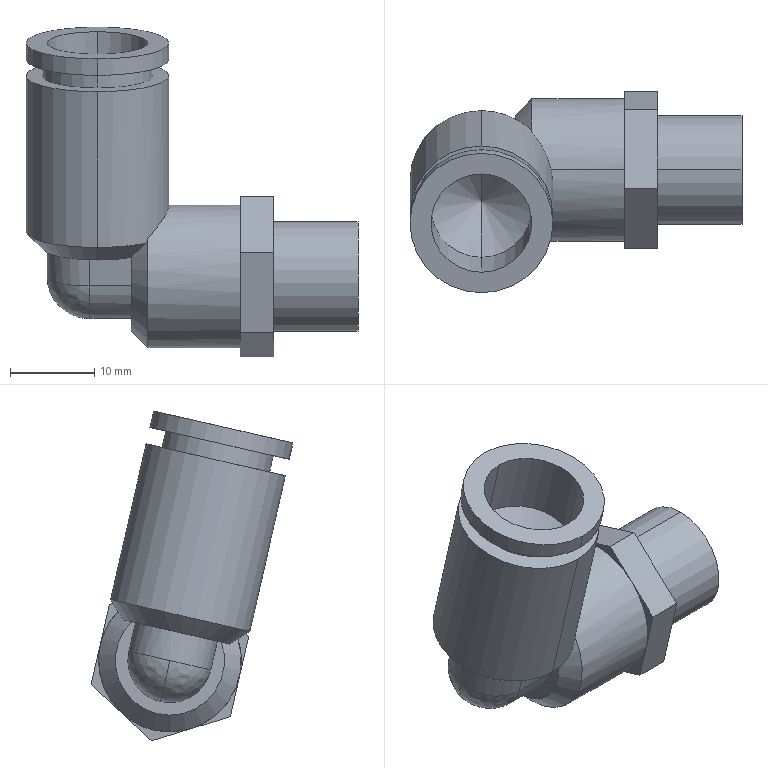Part | SolidWorks | features BaseBody 1 | 1 solid | 44 faces | box 39.5 x 24.022 x 39.246 mm | volume 10032 mm3 | plane 21 | cylinder 14 | cone 7 | spline 2 | commonest cylinder face diameters 17 x6 10 x2 12 x2 13 x2 13.143 x2
STEP:
#1=CARTESIAN_POINT('',(-321.521,1913.544,-45.));
#2=VERTEX_POINT('',#1);
#3=CARTESIAN_POINT('',(-316.521,1908.67,-46.115));
#4=VERTEX_POINT('',#3);
#5=CARTESIAN_POINT('',(-316.521,1913.544,-45.));
#6=DIRECTION('',(0.,-0.223,0.9748));
#7=DIRECTION('',(0.,0.9748,0.223));
#8=AXIS2_PLACEMENT_3D('',#5,#6,#7);
#9=CIRCLE('',#8,5.);
#10=EDGE_CURVE('',#2,#4,#9,.T.);
#11=ORIENTED_EDGE('',*,*,#10,.F.);
#12=CARTESIAN_POINT('',(-316.521,1914.659,-49.874));
#13=VERTEX_POINT('',#12);
#14=CARTESIAN_POINT('',(-316.521,1913.544,-45.));
#15=DIRECTION('',(0.,-0.9748,-0.223));
#16=DIRECTION('',(0.,-0.223,0.9748));
#17=AXIS2_PLACEMENT_3D('',#14,#15,#16);
#18=CIRCLE('',#17,5.);
#19=EDGE_CURVE('',#2,#13,#18,.T.);
#20=ORIENTED_EDGE('',*,*,#19,.T.);
#21=CARTESIAN_POINT('',(-316.521,1913.544,-45.));
#22=DIRECTION('',(1.,0.,0.));
#23=DIRECTION('',(0.,0.,1.));
#24=AXIS2_PLACEMENT_3D('',#21,#22,#23);
#25=CIRCLE('',#24,5.);
#26=EDGE_CURVE('',#4,#13,#25,.T.);
#27=ORIENTED_EDGE('',*,*,#26,.F.);
#28=EDGE_LOOP('',(#11,#20,#27));
#29=FACE_OUTER_BOUND('',#28,.T.);
#30=CARTESIAN_POINT('',(-321.521,1913.544,-45.));
#31=CARTESIAN_POINT('',(-321.521,1910.689,-45.653));
#32=CARTESIAN_POINT('',(-319.45,1908.67,-46.115));
#33=CARTESIAN_POINT('',(-316.521,1908.67,-46.115));
#34=CARTESIAN_POINT('',(-321.521,1914.197,-47.855));
#35=CARTESIAN_POINT('',(-321.521,1911.342,-48.508));
#36=CARTESIAN_POINT('',(-319.45,1909.323,-48.97));
#37=CARTESIAN_POINT('',(-316.521,1909.323,-48.97));
#38=CARTESIAN_POINT('',(-319.45,1914.659,-49.874));
#39=CARTESIAN_POINT('',(-319.45,1912.987,-50.257));
#40=CARTESIAN_POINT('',(-318.237,1911.804,-50.527));
#41=CARTESIAN_POINT('',(-316.521,1911.804,-50.527));
#42=CARTESIAN_POINT('',(-316.521,1914.659,-49.874));
#43=CARTESIAN_POINT('',(-316.521,1914.659,-49.874));
#44=CARTESIAN_POINT('',(-316.521,1914.659,-49.874));
#45=CARTESIAN_POINT('',(-316.521,1914.659,-49.874));
#46=(BOUNDED_SURFACE()B_SPLINE_SURFACE(3,3,((#30,#31,#32,#33),(#34,#35,#36,#37),(#38,#39,#40,#41),(#42,#43,#44,#45)),.UNSPECIFIED.,.F.,.F.,.F.)B_SPLINE_SURFACE_WITH_KNOTS((4,4),(4,4),(0.,1.),(0.,1.),.UNSPECIFIED.)GEOMETRIC_REPRESENTATION_ITEM()RATIONAL_B_SPLINE_SURFACE(((1.,0.8047,0.8047,1.),(0.8047,0.6476,0.6476,0.8047),(0.8047,0.6476,0.6476,0.8047),(1.,0.8047,0.8047,1.)))REPRESENTATION_ITEM('')SURFACE());
#47=ADVANCED_FACE('',(#29),#46,.T.);
#48=CARTESIAN_POINT('',(-315.521,1916.366,-19.221));
#49=VERTEX_POINT('',#48);
#50=CARTESIAN_POINT('',(-315.521,1899.794,-23.013));
#51=VERTEX_POINT('',#50);
#52=CARTESIAN_POINT('',(-315.521,1908.08,-21.117));
#53=DIRECTION('',(0.,0.223,-0.9748));
#54=DIRECTION('',(0.,0.9748,0.223));
#55=AXIS2_PLACEMENT_3D('',#52,#53,#54);
#56=CIRCLE('',#55,8.5);
#57=EDGE_CURVE('',#49,#51,#56,.T.);
#58=ORIENTED_EDGE('',*,*,#57,.T.);
#59=CARTESIAN_POINT('',(-315.521,1904.032,-41.534));
#60=VERTEX_POINT('',#59);
#61=CARTESIAN_POINT('',(-315.521,1898.902,-19.113));
#62=DIRECTION('',(0.,0.223,-0.9748));
#63=VECTOR('',#62,1000.);
#64=LINE('',#61,#63);
#65=EDGE_CURVE('',#51,#60,#64,.T.);
#66=ORIENTED_EDGE('',*,*,#65,.T.);
#67=CARTESIAN_POINT('',(-309.722,1906.259,-41.024));
#68=VERTEX_POINT('',#67);
#69=CARTESIAN_POINT('',(-315.521,1912.317,-39.639));
#70=DIRECTION('',(0.,-0.223,0.9748));
#71=DIRECTION('',(0.,0.9748,0.223));
#72=AXIS2_PLACEMENT_3D('',#69,#70,#71);
#73=CIRCLE('',#72,8.5);
#74=EDGE_CURVE('',#60,#68,#73,.T.);
#75=ORIENTED_EDGE('',*,*,#74,.T.);
#76=CARTESIAN_POINT('',(-309.521,1906.337,-40.494));
#77=VERTEX_POINT('',#76);
#78=CARTESIAN_POINT('',(-309.722,1906.259,-41.024));
#79=CARTESIAN_POINT('',(-309.657,1906.281,-40.847));
#80=CARTESIAN_POINT('',(-309.589,1906.307,-40.67));
#81=CARTESIAN_POINT('',(-309.521,1906.337,-40.494));
#82=B_SPLINE_CURVE_WITH_KNOTS('',3,(#78,#79,#80,#81),.UNSPECIFIED.,.F.,.F.,(4,4),(0.,0.0005727),.UNSPECIFIED.);
#83=EDGE_CURVE('',#68,#77,#82,.T.);
#84=ORIENTED_EDGE('',*,*,#83,.T.);
#85=CARTESIAN_POINT('',(-307.235,1913.544,-36.5));
#86=VERTEX_POINT('',#85);
#87=CARTESIAN_POINT('',(-309.521,1906.337,-40.494));
#88=CARTESIAN_POINT('',(-307.398,1907.926,-37.953));
#89=CARTESIAN_POINT('',(-306.567,1910.547,-36.5));
#90=CARTESIAN_POINT('',(-307.235,1913.544,-36.5));
#91=(BOUNDED_CURVE()B_SPLINE_CURVE(3,(#87,#88,#89,#90),.UNSPECIFIED.,.F.,.F.)B_SPLINE_CURVE_WITH_KNOTS((4,4),(2.354,3.366),.UNSPECIFIED.)CURVE()GEOMETRIC_REPRESENTATION_ITEM()RATIONAL_B_SPLINE_CURVE((1.,0.9165,0.9165,1.))REPRESENTATION_ITEM(''));
#92=EDGE_CURVE('',#77,#86,#91,.T.);
#93=ORIENTED_EDGE('',*,*,#92,.T.);
#94=CARTESIAN_POINT('',(-309.521,1918.075,-37.808));
#95=VERTEX_POINT('',#94);
#96=CARTESIAN_POINT('',(-307.235,1913.544,-36.5));
#97=CARTESIAN_POINT('',(-307.595,1915.158,-36.5));
#98=CARTESIAN_POINT('',(-308.378,1916.709,-36.948));
#99=CARTESIAN_POINT('',(-309.521,1918.075,-37.808));
#100=(BOUNDED_CURVE()B_SPLINE_CURVE(3,(#96,#97,#98,#99),.UNSPECIFIED.,.F.,.F.)B_SPLINE_CURVE_WITH_KNOTS((4,4),(3.366,3.929),.UNSPECIFIED.)CURVE()GEOMETRIC_REPRESENTATION_ITEM()RATIONAL_B_SPLINE_CURVE((1.,0.9738,0.9738,1.))REPRESENTATION_ITEM(''));
#101=EDGE_CURVE('',#86,#95,#100,.T.);
#102=ORIENTED_EDGE('',*,*,#101,.T.);
#103=CARTESIAN_POINT('',(-309.722,1918.376,-38.253));
#104=VERTEX_POINT('',#103);
#105=CARTESIAN_POINT('',(-309.521,1918.075,-37.808));
#106=CARTESIAN_POINT('',(-309.589,1918.178,-37.954));
#107=CARTESIAN_POINT('',(-309.657,1918.278,-38.102));
#108=CARTESIAN_POINT('',(-309.722,1918.376,-38.253));
#109=B_SPLINE_CURVE_WITH_KNOTS('',3,(#105,#106,#107,#108),.UNSPECIFIED.,.F.,.F.,(4,4),(0.,0.0005727),.UNSPECIFIED.);
#110=EDGE_CURVE('',#95,#104,#109,.T.);
#111=ORIENTED_EDGE('',*,*,#110,.T.);
#112=CARTESIAN_POINT('',(-315.521,1920.603,-37.743));
#113=VERTEX_POINT('',#112);
#114=CARTESIAN_POINT('',(-315.521,1912.317,-39.639));
#115=DIRECTION('',(0.,-0.223,0.9748));
#116=DIRECTION('',(0.,0.9748,0.223));
#117=AXIS2_PLACEMENT_3D('',#114,#115,#116);
#118=CIRCLE('',#117,8.5);
#119=EDGE_CURVE('',#104,#113,#118,.T.);
#120=ORIENTED_EDGE('',*,*,#119,.T.);
#121=CARTESIAN_POINT('',(-315.521,1915.474,-15.322));
#122=DIRECTION('',(0.,0.223,-0.9748));
#123=VECTOR('',#122,1000.);
#124=LINE('',#121,#123);
#125=EDGE_CURVE('',#49,#113,#124,.T.);
#126=ORIENTED_EDGE('',*,*,#125,.F.);
#127=EDGE_LOOP('',(#58,#66,#75,#84,#93,#102,#111,#120,#126));
#128=FACE_OUTER_BOUND('',#127,.T.);
#129=CARTESIAN_POINT('',(-315.521,1907.188,-17.218));
#130=DIRECTION('',(0.,0.223,-0.9748));
#131=DIRECTION('',(0.,0.9748,0.223));
#132=AXIS2_PLACEMENT_3D('',#129,#130,#131);
#133=CYLINDRICAL_SURFACE('',#132,8.5);
#134=ADVANCED_FACE('',(#128),#133,.T.);
#135=CARTESIAN_POINT('',(-298.521,1919.329,-51.228));
#136=VERTEX_POINT('',#135);
#137=CARTESIAN_POINT('',(-298.521,1913.544,-53.5));
#138=VERTEX_POINT('',#137);
#139=CARTESIAN_POINT('',(-298.521,1913.544,-45.));
#140=DIRECTION('',(-1.,0.,0.));
#141=DIRECTION('',(0.,0.,1.));
#142=AXIS2_PLACEMENT_3D('',#139,#140,#141);
#143=CIRCLE('',#142,8.5);
#144=EDGE_CURVE('',#136,#138,#143,.T.);
#145=ORIENTED_EDGE('',*,*,#144,.T.);
#146=CARTESIAN_POINT('',(-309.521,1913.544,-53.5));
#147=VERTEX_POINT('',#146);
#148=CARTESIAN_POINT('',(-298.521,1913.544,-53.5));
#149=DIRECTION('',(-1.,0.,0.));
#150=VECTOR('',#149,1000.);
#151=LINE('',#148,#150);
#152=EDGE_CURVE('',#138,#147,#151,.T.);
#153=ORIENTED_EDGE('',*,*,#152,.T.);
#154=CARTESIAN_POINT('',(-309.521,1913.544,-45.));
#155=DIRECTION('',(1.,0.,0.));
#156=DIRECTION('',(0.,0.,1.));
#157=AXIS2_PLACEMENT_3D('',#154,#155,#156);
#158=CIRCLE('',#157,8.5);
#159=EDGE_CURVE('',#147,#95,#158,.T.);
#160=ORIENTED_EDGE('',*,*,#159,.T.);
#161=ORIENTED_EDGE('',*,*,#101,.F.);
#162=CARTESIAN_POINT('',(-298.521,1913.544,-36.5));
#163=VERTEX_POINT('',#162);
#164=CARTESIAN_POINT('',(-298.521,1913.544,-36.5));
#165=DIRECTION('',(-1.,0.,0.));
#166=VECTOR('',#165,1000.);
#167=LINE('',#164,#166);
#168=EDGE_CURVE('',#163,#86,#167,.T.);
#169=ORIENTED_EDGE('',*,*,#168,.F.);
#170=CARTESIAN_POINT('',(-298.521,1916.045,-36.876));
#171=VERTEX_POINT('',#170);
#172=CARTESIAN_POINT('',(-298.521,1913.544,-45.));
#173=DIRECTION('',(-1.,0.,0.));
#174=DIRECTION('',(0.,0.,1.));
#175=AXIS2_PLACEMENT_3D('',#172,#173,#174);
#176=CIRCLE('',#175,8.5);
#177=EDGE_CURVE('',#163,#171,#176,.T.);
#178=ORIENTED_EDGE('',*,*,#177,.T.);
#179=CARTESIAN_POINT('',(-298.521,1921.83,-43.104));
#180=VERTEX_POINT('',#179);
#181=CARTESIAN_POINT('',(-298.521,1913.544,-45.));
#182=DIRECTION('',(-1.,0.,0.));
#183=DIRECTION('',(0.,0.,1.));
#184=AXIS2_PLACEMENT_3D('',#181,#182,#183);
#185=CIRCLE('',#184,8.5);
#186=EDGE_CURVE('',#171,#180,#185,.T.);
#187=ORIENTED_EDGE('',*,*,#186,.T.);
#188=CARTESIAN_POINT('',(-298.521,1913.544,-45.));
#189=DIRECTION('',(-1.,0.,0.));
#190=DIRECTION('',(0.,0.,1.));
#191=AXIS2_PLACEMENT_3D('',#188,#189,#190);
#192=CIRCLE('',#191,8.5);
#193=EDGE_CURVE('',#180,#136,#192,.T.);
#194=ORIENTED_EDGE('',*,*,#193,.T.);
#195=EDGE_LOOP('',(#145,#153,#160,#161,#169,#178,#187,#194));
#196=FACE_OUTER_BOUND('',#195,.T.);
#197=CARTESIAN_POINT('',(-298.521,1913.544,-45.));
#198=DIRECTION('',(-1.,0.,0.));
#199=DIRECTION('',(0.,0.,1.));
#200=AXIS2_PLACEMENT_3D('',#197,#198,#199);
#201=CYLINDRICAL_SURFACE('',#200,8.5);
#202=ADVANCED_FACE('',(#196),#201,.T.);
#203=CARTESIAN_POINT('',(-311.521,1917.758,-40.446));
#204=VERTEX_POINT('',#203);
#205=CARTESIAN_POINT('',(-315.521,1919.1,-40.139));
#206=VERTEX_POINT('',#205);
#207=CARTESIAN_POINT('',(-315.521,1912.763,-41.588));
#208=DIRECTION('',(0.,-0.223,0.9748));
#209=DIRECTION('',(0.,-0.9748,-0.223));
#210=AXIS2_PLACEMENT_3D('',#207,#208,#209);
#211=CIRCLE('',#210,6.5);
#212=EDGE_CURVE('',#204,#206,#211,.T.);
#213=ORIENTED_EDGE('',*,*,#212,.T.);
#214=CARTESIAN_POINT('',(-315.521,1920.603,-37.743));
#215=DIRECTION('',(0.,0.5316,0.847));
#216=VECTOR('',#215,1000.);
#217=LINE('',#214,#216);
#218=EDGE_CURVE('',#206,#113,#217,.T.);
#219=ORIENTED_EDGE('',*,*,#218,.T.);
#220=ORIENTED_EDGE('',*,*,#119,.F.);
#221=CARTESIAN_POINT('',(-311.521,1917.943,-40.214));
#222=VERTEX_POINT('',#221);
#223=CARTESIAN_POINT('',(-309.722,1918.376,-38.253));
#224=CARTESIAN_POINT('',(-310.327,1918.25,-38.906));
#225=CARTESIAN_POINT('',(-310.927,1918.108,-39.56));
#226=CARTESIAN_POINT('',(-311.521,1917.943,-40.214));
#227=B_SPLINE_CURVE_WITH_KNOTS('',3,(#223,#224,#225,#226),.UNSPECIFIED.,.F.,.F.,(4,4),(0.,0.002697),.UNSPECIFIED.);
#228=EDGE_CURVE('',#104,#222,#227,.T.);
#229=ORIENTED_EDGE('',*,*,#228,.T.);
#230=CARTESIAN_POINT('',(-311.521,1917.943,-40.214));
#231=CARTESIAN_POINT('',(-311.521,1917.881,-40.292));
#232=CARTESIAN_POINT('',(-311.521,1917.82,-40.369));
#233=CARTESIAN_POINT('',(-311.521,1917.758,-40.446));
#234=B_SPLINE_CURVE_WITH_KNOTS('',3,(#230,#231,#232,#233),.UNSPECIFIED.,.F.,.F.,(4,4),(0.,0.0002959),.UNSPECIFIED.);
#235=EDGE_CURVE('',#222,#204,#234,.T.);
#236=ORIENTED_EDGE('',*,*,#235,.T.);
#237=EDGE_LOOP('',(#213,#219,#220,#229,#236));
#238=FACE_OUTER_BOUND('',#237,.T.);
#239=CARTESIAN_POINT('',(-315.521,1912.317,-39.639));
#240=DIRECTION('',(0.,-0.223,0.9748));
#241=DIRECTION('',(0.,-0.9748,-0.223));
#242=AXIS2_PLACEMENT_3D('',#239,#240,#241);
#243=CONICAL_SURFACE('',#242,8.5,0.7854);
#244=ADVANCED_FACE('',(#238),#243,.T.);
#245=ORIENTED_EDGE('',*,*,#218,.F.);
#246=CARTESIAN_POINT('',(-315.521,1906.427,-43.038));
#247=VERTEX_POINT('',#246);
#248=CARTESIAN_POINT('',(-315.521,1912.763,-41.588));
#249=DIRECTION('',(0.,-0.223,0.9748));
#250=DIRECTION('',(0.,-0.9748,-0.223));
#251=AXIS2_PLACEMENT_3D('',#248,#249,#250);
#252=CIRCLE('',#251,6.5);
#253=EDGE_CURVE('',#206,#247,#252,.T.);
#254=ORIENTED_EDGE('',*,*,#253,.T.);
#255=CARTESIAN_POINT('',(-315.521,1904.032,-41.534));
#256=DIRECTION('',(0.,-0.847,0.5316));
#257=VECTOR('',#256,1000.);
#258=LINE('',#255,#257);
#259=EDGE_CURVE('',#247,#60,#258,.T.);
#260=ORIENTED_EDGE('',*,*,#259,.T.);
#261=CARTESIAN_POINT('',(-315.521,1912.317,-39.639));
#262=DIRECTION('',(0.,-0.223,0.9748));
#263=DIRECTION('',(0.,0.9748,0.223));
#264=AXIS2_PLACEMENT_3D('',#261,#262,#263);
#265=CIRCLE('',#264,8.5);
#266=EDGE_CURVE('',#113,#60,#265,.T.);
#267=ORIENTED_EDGE('',*,*,#266,.F.);
#268=EDGE_LOOP('',(#245,#254,#260,#267));
#269=FACE_OUTER_BOUND('',#268,.T.);
#270=CARTESIAN_POINT('',(-315.521,1912.317,-39.639));
#271=DIRECTION('',(0.,-0.223,0.9748));
#272=DIRECTION('',(0.,-0.9748,-0.223));
#273=AXIS2_PLACEMENT_3D('',#270,#271,#272);
#274=CONICAL_SURFACE('',#273,8.5,0.7854);
#275=ADVANCED_FACE('',(#269),#274,.T.);
#276=CARTESIAN_POINT('',(-311.521,1907.502,-42.603));
#277=VERTEX_POINT('',#276);
#278=CARTESIAN_POINT('',(-311.521,1913.544,-51.5));
#279=VERTEX_POINT('',#278);
#280=CARTESIAN_POINT('',(-311.521,1913.544,-45.));
#281=DIRECTION('',(1.,0.,0.));
#282=DIRECTION('',(0.,0.,-1.));
#283=AXIS2_PLACEMENT_3D('',#280,#281,#282);
#284=CIRCLE('',#283,6.5);
#285=EDGE_CURVE('',#277,#279,#284,.T.);
#286=ORIENTED_EDGE('',*,*,#285,.T.);
#287=CARTESIAN_POINT('',(-309.521,1913.544,-53.5));
#288=DIRECTION('',(0.7071,0.,-0.7071));
#289=VECTOR('',#288,1000.);
#290=LINE('',#287,#289);
#291=EDGE_CURVE('',#279,#147,#290,.T.);
#292=ORIENTED_EDGE('',*,*,#291,.T.);
#293=CARTESIAN_POINT('',(-309.521,1913.544,-45.));
#294=DIRECTION('',(1.,0.,0.));
#295=DIRECTION('',(0.,0.,1.));
#296=AXIS2_PLACEMENT_3D('',#293,#294,#295);
#297=CIRCLE('',#296,8.5);
#298=EDGE_CURVE('',#77,#147,#297,.T.);
#299=ORIENTED_EDGE('',*,*,#298,.F.);
#300=ORIENTED_EDGE('',*,*,#83,.F.);
#301=CARTESIAN_POINT('',(-311.521,1907.502,-42.603));
#302=CARTESIAN_POINT('',(-310.927,1907.069,-42.085));
#303=CARTESIAN_POINT('',(-310.327,1906.657,-41.558));
#304=CARTESIAN_POINT('',(-309.722,1906.259,-41.024));
#305=B_SPLINE_CURVE_WITH_KNOTS('',3,(#301,#302,#303,#304),.UNSPECIFIED.,.F.,.F.,(4,4),(0.,0.002697),.UNSPECIFIED.);
#306=EDGE_CURVE('',#277,#68,#305,.T.);
#307=ORIENTED_EDGE('',*,*,#306,.F.);
#308=EDGE_LOOP('',(#286,#292,#299,#300,#307));
#309=FACE_OUTER_BOUND('',#308,.T.);
#310=CARTESIAN_POINT('',(-309.521,1913.544,-45.));
#311=DIRECTION('',(1.,0.,0.));
#312=DIRECTION('',(0.,0.,-1.));
#313=AXIS2_PLACEMENT_3D('',#310,#311,#312);
#314=CONICAL_SURFACE('',#313,8.5,0.7854);
#315=ADVANCED_FACE('',(#309),#314,.T.);
#316=CARTESIAN_POINT('',(-315.521,1914.04,-17.702));
#317=VERTEX_POINT('',#316);
#318=CARTESIAN_POINT('',(-315.521,1901.228,-20.633));
#319=VERTEX_POINT('',#318);
#320=CARTESIAN_POINT('',(-315.521,1907.634,-19.167));
#321=DIRECTION('',(0.,0.223,-0.9748));
#322=DIRECTION('',(0.,0.9748,0.223));
#323=AXIS2_PLACEMENT_3D('',#320,#321,#322);
#324=CIRCLE('',#323,6.571);
#325=EDGE_CURVE('',#317,#319,#324,.T.);
#326=ORIENTED_EDGE('',*,*,#325,.T.);
#327=CARTESIAN_POINT('',(-315.521,1901.674,-22.583));
#328=VERTEX_POINT('',#327);
#329=CARTESIAN_POINT('',(-315.521,1901.451,-21.608));
#330=DIRECTION('',(0.,0.223,-0.9748));
#331=VECTOR('',#330,1000.);
#332=LINE('',#329,#331);
#333=EDGE_CURVE('',#319,#328,#332,.T.);
#334=ORIENTED_EDGE('',*,*,#333,.T.);
#335=CARTESIAN_POINT('',(-315.521,1914.486,-19.652));
#336=VERTEX_POINT('',#335);
#337=CARTESIAN_POINT('',(-315.521,1908.08,-21.117));
#338=DIRECTION('',(0.,-0.223,0.9748));
#339=DIRECTION('',(0.,0.9748,0.223));
#340=AXIS2_PLACEMENT_3D('',#337,#338,#339);
#341=CIRCLE('',#340,6.571);
#342=EDGE_CURVE('',#328,#336,#341,.T.);
#343=ORIENTED_EDGE('',*,*,#342,.T.);
#344=CARTESIAN_POINT('',(-315.521,1914.263,-18.677));
#345=DIRECTION('',(0.,0.223,-0.9748));
#346=VECTOR('',#345,1000.);
#347=LINE('',#344,#346);
#348=EDGE_CURVE('',#317,#336,#347,.T.);
#349=ORIENTED_EDGE('',*,*,#348,.F.);
#350=EDGE_LOOP('',(#326,#334,#343,#349));
#351=FACE_OUTER_BOUND('',#350,.T.);
#352=CARTESIAN_POINT('',(-315.521,1907.857,-20.142));
#353=DIRECTION('',(0.,0.223,-0.9748));
#354=DIRECTION('',(0.,0.9748,0.223));
#355=AXIS2_PLACEMENT_3D('',#352,#353,#354);
#356=CYLINDRICAL_SURFACE('',#355,6.571);
#357=ADVANCED_FACE('',(#351),#356,.T.);
#358=CARTESIAN_POINT('',(-315.521,1915.474,-15.322));
#359=VERTEX_POINT('',#358);
#360=CARTESIAN_POINT('',(-315.521,1898.902,-19.113));
#361=VERTEX_POINT('',#360);
#362=CARTESIAN_POINT('',(-315.521,1907.188,-17.218));
#363=DIRECTION('',(0.,0.223,-0.9748));
#364=DIRECTION('',(0.,0.9748,0.223));
#365=AXIS2_PLACEMENT_3D('',#362,#363,#364);
#366=CIRCLE('',#365,8.5);
#367=EDGE_CURVE('',#359,#361,#366,.T.);
#368=ORIENTED_EDGE('',*,*,#367,.T.);
#369=CARTESIAN_POINT('',(-315.521,1899.348,-21.063));
#370=VERTEX_POINT('',#369);
#371=CARTESIAN_POINT('',(-315.521,1898.902,-19.113));
#372=DIRECTION('',(0.,0.223,-0.9748));
#373=VECTOR('',#372,1000.);
#374=LINE('',#371,#373);
#375=EDGE_CURVE('',#361,#370,#374,.T.);
#376=ORIENTED_EDGE('',*,*,#375,.T.);
#377=CARTESIAN_POINT('',(-315.521,1915.92,-17.272));
#378=VERTEX_POINT('',#377);
#379=CARTESIAN_POINT('',(-315.521,1907.634,-19.167));
#380=DIRECTION('',(0.,-0.223,0.9748));
#381=DIRECTION('',(0.,0.9748,0.223));
#382=AXIS2_PLACEMENT_3D('',#379,#380,#381);
#383=CIRCLE('',#382,8.5);
#384=EDGE_CURVE('',#370,#378,#383,.T.);
#385=ORIENTED_EDGE('',*,*,#384,.T.);
#386=CARTESIAN_POINT('',(-315.521,1915.474,-15.322));
#387=DIRECTION('',(0.,0.223,-0.9748));
#388=VECTOR('',#387,1000.);
#389=LINE('',#386,#388);
#390=EDGE_CURVE('',#359,#378,#389,.T.);
#391=ORIENTED_EDGE('',*,*,#390,.F.);
#392=EDGE_LOOP('',(#368,#376,#385,#391));
#393=FACE_OUTER_BOUND('',#392,.T.);
#394=CARTESIAN_POINT('',(-315.521,1907.188,-17.218));
#395=DIRECTION('',(0.,0.223,-0.9748));
#396=DIRECTION('',(0.,0.9748,0.223));
#397=AXIS2_PLACEMENT_3D('',#394,#395,#396);
#398=CYLINDRICAL_SURFACE('',#397,8.5);
#399=ADVANCED_FACE('',(#393),#398,.T.);
#400=CARTESIAN_POINT('',(-294.521,1913.544,-51.5));
#401=VERTEX_POINT('',#400);
#402=CARTESIAN_POINT('',(-294.521,1913.544,-38.5));
#403=VERTEX_POINT('',#402);
#404=CARTESIAN_POINT('',(-294.521,1913.544,-45.));
#405=DIRECTION('',(1.,0.,0.));
#406=DIRECTION('',(0.,0.,-1.));
#407=AXIS2_PLACEMENT_3D('',#404,#405,#406);
#408=CIRCLE('',#407,6.5);
#409=EDGE_CURVE('',#401,#403,#408,.T.);
#410=ORIENTED_EDGE('',*,*,#409,.T.);
#411=CARTESIAN_POINT('',(-284.521,1913.544,-38.5));
#412=VERTEX_POINT('',#411);
#413=CARTESIAN_POINT('',(-294.521,1913.544,-38.5));
#414=DIRECTION('',(1.,0.,0.));
#415=VECTOR('',#414,1000.);
#416=LINE('',#413,#415);
#417=EDGE_CURVE('',#403,#412,#416,.T.);
#418=ORIENTED_EDGE('',*,*,#417,.T.);
#419=CARTESIAN_POINT('',(-284.521,1913.544,-51.5));
#420=VERTEX_POINT('',#419);
#421=CARTESIAN_POINT('',(-284.521,1913.544,-45.));
#422=DIRECTION('',(-1.,0.,0.));
#423=DIRECTION('',(0.,0.,-1.));
#424=AXIS2_PLACEMENT_3D('',#421,#422,#423);
#425=CIRCLE('',#424,6.5);
#426=EDGE_CURVE('',#412,#420,#425,.T.);
#427=ORIENTED_EDGE('',*,*,#426,.T.);
#428=CARTESIAN_POINT('',(-294.521,1913.544,-51.5));
#429=DIRECTION('',(1.,0.,0.));
#430=VECTOR('',#429,1000.);
#431=LINE('',#428,#430);
#432=EDGE_CURVE('',#401,#420,#431,.T.);
#433=ORIENTED_EDGE('',*,*,#432,.F.);
#434=EDGE_LOOP('',(#410,#418,#427,#433));
#435=FACE_OUTER_BOUND('',#434,.T.);
#436=CARTESIAN_POINT('',(-294.521,1913.544,-45.));
#437=DIRECTION('',(1.,0.,0.));
#438=DIRECTION('',(0.,0.,-1.));
#439=AXIS2_PLACEMENT_3D('',#436,#437,#438);
#440=CYLINDRICAL_SURFACE('',#439,6.5);
#441=ADVANCED_FACE('',(#435),#440,.T.);
#442=CARTESIAN_POINT('',(-315.521,1914.821,-23.678));
#443=VERTEX_POINT('',#442);
#444=CARTESIAN_POINT('',(-315.521,1903.123,-26.354));
#445=VERTEX_POINT('',#444);
#446=CARTESIAN_POINT('',(-315.521,1908.972,-25.016));
#447=DIRECTION('',(0.,-0.223,0.9748));
#448=DIRECTION('',(0.,-0.9748,-0.223));
#449=AXIS2_PLACEMENT_3D('',#446,#447,#448);
#450=CIRCLE('',#449,6.);
#451=EDGE_CURVE('',#443,#445,#450,.T.);
#452=ORIENTED_EDGE('',*,*,#451,.F.);
#453=CARTESIAN_POINT('',(-315.521,1913.037,-15.88));
#454=VERTEX_POINT('',#453);
#455=CARTESIAN_POINT('',(-315.521,1913.929,-19.779));
#456=DIRECTION('',(0.,-0.223,0.9748));
#457=VECTOR('',#456,1000.);
#458=LINE('',#455,#457);
#459=EDGE_CURVE('',#443,#454,#458,.T.);
#460=ORIENTED_EDGE('',*,*,#459,.T.);
#461=CARTESIAN_POINT('',(-315.521,1901.339,-18.556));
#462=VERTEX_POINT('',#461);
#463=CARTESIAN_POINT('',(-315.521,1907.188,-17.218));
#464=DIRECTION('',(0.,-0.223,0.9748));
#465=DIRECTION('',(0.,-0.9748,-0.223));
#466=AXIS2_PLACEMENT_3D('',#463,#464,#465);
#467=CIRCLE('',#466,6.);
#468=EDGE_CURVE('',#454,#462,#467,.T.);
#469=ORIENTED_EDGE('',*,*,#468,.T.);
#470=CARTESIAN_POINT('',(-315.521,1902.231,-22.455));
#471=DIRECTION('',(0.,-0.223,0.9748));
#472=VECTOR('',#471,1000.);
#473=LINE('',#470,#472);
#474=EDGE_CURVE('',#445,#462,#473,.T.);
#475=ORIENTED_EDGE('',*,*,#474,.F.);
#476=EDGE_LOOP('',(#452,#460,#469,#475));
#477=FACE_OUTER_BOUND('',#476,.T.);
#478=CARTESIAN_POINT('',(-315.521,1908.08,-21.117));
#479=DIRECTION('',(0.,-0.223,0.9748));
#480=DIRECTION('',(0.,-0.9748,-0.223));
#481=AXIS2_PLACEMENT_3D('',#478,#479,#480);
#482=CYLINDRICAL_SURFACE('',#481,6.);
#483=ADVANCED_FACE('',(#477),#482,.F.);
#484=CARTESIAN_POINT('',(-315.521,1909.776,-28.531));
#485=VERTEX_POINT('',#484);
#486=CARTESIAN_POINT('',(-315.521,1903.123,-26.354));
#487=DIRECTION('',(0.,-0.9504,0.3109));
#488=VECTOR('',#487,1000.);
#489=LINE('',#486,#488);
#490=EDGE_CURVE('',#485,#445,#489,.T.);
#491=ORIENTED_EDGE('',*,*,#490,.F.);
#492=CARTESIAN_POINT('',(-315.521,1914.821,-23.678));
#493=DIRECTION('',(0.,0.7207,0.6932));
#494=VECTOR('',#493,1000.);
#495=LINE('',#492,#494);
#496=EDGE_CURVE('',#485,#443,#495,.T.);
#497=ORIENTED_EDGE('',*,*,#496,.T.);
#498=ORIENTED_EDGE('',*,*,#451,.T.);
#499=EDGE_LOOP('',(#491,#497,#498));
#500=FACE_OUTER_BOUND('',#499,.T.);
#501=CARTESIAN_POINT('',(-315.521,1908.972,-25.016));
#502=DIRECTION('',(0.,-0.223,0.9748));
#503=DIRECTION('',(0.,-0.9748,-0.223));
#504=AXIS2_PLACEMENT_3D('',#501,#502,#503);
#505=CONICAL_SURFACE('',#504,6.,1.03);
#506=ADVANCED_FACE('',(#500),#505,.F.);
#507=ORIENTED_EDGE('',*,*,#65,.F.);
#508=CARTESIAN_POINT('',(-315.521,1908.08,-21.117));
#509=DIRECTION('',(0.,0.223,-0.9748));
#510=DIRECTION('',(0.,0.9748,0.223));
#511=AXIS2_PLACEMENT_3D('',#508,#509,#510);
#512=CIRCLE('',#511,8.5);
#513=EDGE_CURVE('',#51,#49,#512,.T.);
#514=ORIENTED_EDGE('',*,*,#513,.T.);
#515=ORIENTED_EDGE('',*,*,#125,.T.);
#516=ORIENTED_EDGE('',*,*,#266,.T.);
#517=EDGE_LOOP('',(#507,#514,#515,#516));
#518=FACE_OUTER_BOUND('',#517,.T.);
#519=CARTESIAN_POINT('',(-315.521,1907.188,-17.218));
#520=DIRECTION('',(0.,0.223,-0.9748));
#521=DIRECTION('',(0.,0.9748,0.223));
#522=AXIS2_PLACEMENT_3D('',#519,#520,#521);
#523=CYLINDRICAL_SURFACE('',#522,8.5);
#524=ADVANCED_FACE('',(#518),#523,.T.);
#525=ORIENTED_EDGE('',*,*,#152,.F.);
#526=CARTESIAN_POINT('',(-298.521,1911.043,-53.124));
#527=VERTEX_POINT('',#526);
#528=CARTESIAN_POINT('',(-298.521,1913.544,-45.));
#529=DIRECTION('',(-1.,0.,0.));
#530=DIRECTION('',(0.,0.,1.));
#531=AXIS2_PLACEMENT_3D('',#528,#529,#530);
#532=CIRCLE('',#531,8.5);
#533=EDGE_CURVE('',#138,#527,#532,.T.);
#534=ORIENTED_EDGE('',*,*,#533,.T.);
#535=CARTESIAN_POINT('',(-298.521,1905.258,-46.896));
#536=VERTEX_POINT('',#535);
#537=CARTESIAN_POINT('',(-298.521,1913.544,-45.));
#538=DIRECTION('',(-1.,0.,0.));
#539=DIRECTION('',(0.,0.,1.));
#540=AXIS2_PLACEMENT_3D('',#537,#538,#539);
#541=CIRCLE('',#540,8.5);
#542=EDGE_CURVE('',#527,#536,#541,.T.);
#543=ORIENTED_EDGE('',*,*,#542,.T.);
#544=CARTESIAN_POINT('',(-298.521,1907.759,-38.772));
#545=VERTEX_POINT('',#544);
#546=CARTESIAN_POINT('',(-298.521,1913.544,-45.));
#547=DIRECTION('',(-1.,0.,0.));
#548=DIRECTION('',(0.,0.,1.));
#549=AXIS2_PLACEMENT_3D('',#546,#547,#548);
#550=CIRCLE('',#549,8.5);
#551=EDGE_CURVE('',#536,#545,#550,.T.);
#552=ORIENTED_EDGE('',*,*,#551,.T.);
#553=CARTESIAN_POINT('',(-298.521,1913.544,-45.));
#554=DIRECTION('',(-1.,0.,0.));
#555=DIRECTION('',(0.,0.,1.));
#556=AXIS2_PLACEMENT_3D('',#553,#554,#555);
#557=CIRCLE('',#556,8.5);
#558=EDGE_CURVE('',#545,#163,#557,.T.);
#559=ORIENTED_EDGE('',*,*,#558,.T.);
#560=ORIENTED_EDGE('',*,*,#168,.T.);
#561=ORIENTED_EDGE('',*,*,#92,.F.);
#562=ORIENTED_EDGE('',*,*,#298,.T.);
#563=EDGE_LOOP('',(#525,#534,#543,#552,#559,#560,#561,#562));
#564=FACE_OUTER_BOUND('',#563,.T.);
#565=CARTESIAN_POINT('',(-298.521,1913.544,-45.));
#566=DIRECTION('',(-1.,0.,0.));
#567=DIRECTION('',(0.,0.,1.));
#568=AXIS2_PLACEMENT_3D('',#565,#566,#567);
#569=CYLINDRICAL_SURFACE('',#568,8.5);
#570=ADVANCED_FACE('',(#564),#569,.T.);
#571=CARTESIAN_POINT('',(-315.521,1908.08,-21.117));
#572=DIRECTION('',(0.,-0.223,0.9748));
#573=DIRECTION('',(0.,0.9748,0.223));
#574=AXIS2_PLACEMENT_3D('',#571,#572,#573);
#575=CIRCLE('',#574,6.571);
#576=EDGE_CURVE('',#336,#328,#575,.T.);
#577=ORIENTED_EDGE('',*,*,#576,.F.);
#578=ORIENTED_EDGE('',*,*,#342,.F.);
#579=EDGE_LOOP('',(#577,#578));
#580=FACE_BOUND('',#579,.T.);
#581=ORIENTED_EDGE('',*,*,#57,.F.);
#582=ORIENTED_EDGE('',*,*,#513,.F.);
#583=EDGE_LOOP('',(#581,#582));
#584=FACE_OUTER_BOUND('',#583,.T.);
#585=CARTESIAN_POINT('',(-323.092,1908.08,-21.117));
#586=DIRECTION('',(0.,0.223,-0.9748));
#587=DIRECTION('',(0.,0.9748,0.223));
#588=AXIS2_PLACEMENT_3D('',#585,#586,#587);
#589=PLANE('',#588);
#590=ADVANCED_FACE('',(#580,#584),#589,.F.);
#591=ORIENTED_EDGE('',*,*,#259,.F.);
#592=CARTESIAN_POINT('',(-311.521,1907.769,-42.731));
#593=VERTEX_POINT('',#592);
#594=CARTESIAN_POINT('',(-315.521,1912.763,-41.588));
#595=DIRECTION('',(0.,-0.223,0.9748));
#596=DIRECTION('',(0.,-0.9748,-0.223));
#597=AXIS2_PLACEMENT_3D('',#594,#595,#596);
#598=CIRCLE('',#597,6.5);
#599=EDGE_CURVE('',#247,#593,#598,.T.);
#600=ORIENTED_EDGE('',*,*,#599,.T.);
#601=CARTESIAN_POINT('',(-311.521,1907.769,-42.731));
#602=CARTESIAN_POINT('',(-311.521,1907.68,-42.689));
#603=CARTESIAN_POINT('',(-311.521,1907.591,-42.646));
#604=CARTESIAN_POINT('',(-311.521,1907.502,-42.603));
#605=B_SPLINE_CURVE_WITH_KNOTS('',3,(#601,#602,#603,#604),.UNSPECIFIED.,.F.,.F.,(4,4),(0.,0.0002959),.UNSPECIFIED.);
#606=EDGE_CURVE('',#593,#277,#605,.T.);
#607=ORIENTED_EDGE('',*,*,#606,.T.);
#608=ORIENTED_EDGE('',*,*,#306,.T.);
#609=ORIENTED_EDGE('',*,*,#74,.F.);
#610=EDGE_LOOP('',(#591,#600,#607,#608,#609));
#611=FACE_OUTER_BOUND('',#610,.T.);
#612=CARTESIAN_POINT('',(-315.521,1912.317,-39.639));
#613=DIRECTION('',(0.,-0.223,0.9748));
#614=DIRECTION('',(0.,-0.9748,-0.223));
#615=AXIS2_PLACEMENT_3D('',#612,#613,#614);
#616=CONICAL_SURFACE('',#615,8.5,0.7854);
#617=ADVANCED_FACE('',(#611),#616,.T.);
#618=ORIENTED_EDGE('',*,*,#291,.F.);
#619=CARTESIAN_POINT('',(-311.521,1913.544,-45.));
#620=DIRECTION('',(1.,0.,0.));
#621=DIRECTION('',(0.,0.,-1.));
#622=AXIS2_PLACEMENT_3D('',#619,#620,#621);
#623=CIRCLE('',#622,6.5);
#624=EDGE_CURVE('',#279,#222,#623,.T.);
#625=ORIENTED_EDGE('',*,*,#624,.T.);
#626=ORIENTED_EDGE('',*,*,#228,.F.);
#627=ORIENTED_EDGE('',*,*,#110,.F.);
#628=ORIENTED_EDGE('',*,*,#159,.F.);
#629=EDGE_LOOP('',(#618,#625,#626,#627,#628));
#630=FACE_OUTER_BOUND('',#629,.T.);
#631=CARTESIAN_POINT('',(-309.521,1913.544,-45.));
#632=DIRECTION('',(1.,0.,0.));
#633=DIRECTION('',(0.,0.,-1.));
#634=AXIS2_PLACEMENT_3D('',#631,#632,#633);
#635=CONICAL_SURFACE('',#634,8.5,0.7854);
#636=ADVANCED_FACE('',(#630),#635,.T.);
#637=ORIENTED_EDGE('',*,*,#551,.F.);
#638=CARTESIAN_POINT('',(-298.521,1904.164,-42.112));
#639=VERTEX_POINT('',#638);
#640=CARTESIAN_POINT('',(-298.521,1905.258,-46.896));
#641=DIRECTION('',(0.,-0.223,0.9748));
#642=VECTOR('',#641,1000.);
#643=LINE('',#640,#642);
#644=EDGE_CURVE('',#536,#639,#643,.T.);
#645=ORIENTED_EDGE('',*,*,#644,.T.);
#646=CARTESIAN_POINT('',(-298.521,1904.164,-42.112));
#647=DIRECTION('',(0.,0.7327,0.6805));
#648=VECTOR('',#647,1000.);
#649=LINE('',#646,#648);
#650=EDGE_CURVE('',#639,#545,#649,.T.);
#651=ORIENTED_EDGE('',*,*,#650,.T.);
#652=EDGE_LOOP('',(#637,#645,#651));
#653=FACE_OUTER_BOUND('',#652,.T.);
#654=CARTESIAN_POINT('',(-298.521,1913.544,-45.));
#655=DIRECTION('',(-1.,0.,0.));
#656=DIRECTION('',(0.,0.,1.));
#657=AXIS2_PLACEMENT_3D('',#654,#655,#656);
#658=PLANE('',#657);
#659=ADVANCED_FACE('',(#653),#658,.T.);
#660=ORIENTED_EDGE('',*,*,#186,.F.);
#661=CARTESIAN_POINT('',(-298.521,1920.736,-38.321));
#662=VERTEX_POINT('',#661);
#663=CARTESIAN_POINT('',(-298.521,1916.045,-36.876));
#664=DIRECTION('',(0.,0.9557,-0.2943));
#665=VECTOR('',#664,1000.);
#666=LINE('',#663,#665);
#667=EDGE_CURVE('',#171,#662,#666,.T.);
#668=ORIENTED_EDGE('',*,*,#667,.T.);
#669=CARTESIAN_POINT('',(-298.521,1920.736,-38.321));
#670=DIRECTION('',(0.,0.223,-0.9748));
#671=VECTOR('',#670,1000.);
#672=LINE('',#669,#671);
#673=EDGE_CURVE('',#662,#180,#672,.T.);
#674=ORIENTED_EDGE('',*,*,#673,.T.);
#675=EDGE_LOOP('',(#660,#668,#674));
#676=FACE_OUTER_BOUND('',#675,.T.);
#677=CARTESIAN_POINT('',(-298.521,1913.544,-45.));
#678=DIRECTION('',(-1.,0.,0.));
#679=DIRECTION('',(0.,0.,1.));
#680=AXIS2_PLACEMENT_3D('',#677,#678,#679);
#681=PLANE('',#680);
#682=ADVANCED_FACE('',(#676),#681,.T.);
#683=ORIENTED_EDGE('',*,*,#558,.F.);
#684=CARTESIAN_POINT('',(-298.521,1911.355,-35.432));
#685=VERTEX_POINT('',#684);
#686=CARTESIAN_POINT('',(-298.521,1907.759,-38.772));
#687=DIRECTION('',(0.,0.7327,0.6805));
#688=VECTOR('',#687,1000.);
#689=LINE('',#686,#688);
#690=EDGE_CURVE('',#545,#685,#689,.T.);
#691=ORIENTED_EDGE('',*,*,#690,.T.);
#692=CARTESIAN_POINT('',(-298.521,1911.355,-35.432));
#693=DIRECTION('',(0.,0.9557,-0.2943));
#694=VECTOR('',#693,1000.);
#695=LINE('',#692,#694);
#696=EDGE_CURVE('',#685,#171,#695,.T.);
#697=ORIENTED_EDGE('',*,*,#696,.T.);
#698=ORIENTED_EDGE('',*,*,#177,.F.);
#699=EDGE_LOOP('',(#683,#691,#697,#698));
#700=FACE_OUTER_BOUND('',#699,.T.);
#701=CARTESIAN_POINT('',(-298.521,1913.544,-45.));
#702=DIRECTION('',(-1.,0.,0.));
#703=DIRECTION('',(0.,0.,1.));
#704=AXIS2_PLACEMENT_3D('',#701,#702,#703);
#705=PLANE('',#704);
#706=ADVANCED_FACE('',(#700),#705,.T.);
#707=ORIENTED_EDGE('',*,*,#333,.F.);
#708=CARTESIAN_POINT('',(-315.521,1907.634,-19.167));
#709=DIRECTION('',(0.,0.223,-0.9748));
#710=DIRECTION('',(0.,0.9748,0.223));
#711=AXIS2_PLACEMENT_3D('',#708,#709,#710);
#712=CIRCLE('',#711,6.571);
#713=EDGE_CURVE('',#319,#317,#712,.T.);
#714=ORIENTED_EDGE('',*,*,#713,.T.);
#715=ORIENTED_EDGE('',*,*,#348,.T.);
#716=ORIENTED_EDGE('',*,*,#576,.T.);
#717=EDGE_LOOP('',(#707,#714,#715,#716));
#718=FACE_OUTER_BOUND('',#717,.T.);
#719=CARTESIAN_POINT('',(-315.521,1907.857,-20.142));
#720=DIRECTION('',(0.,0.223,-0.9748));
#721=DIRECTION('',(0.,0.9748,0.223));
#722=AXIS2_PLACEMENT_3D('',#719,#720,#721);
#723=CYLINDRICAL_SURFACE('',#722,6.571);
#724=ADVANCED_FACE('',(#718),#723,.T.);
#725=CARTESIAN_POINT('',(-316.521,1917.638,-40.473));
#726=VERTEX_POINT('',#725);
#727=CARTESIAN_POINT('',(-316.521,1907.889,-42.703));
#728=VERTEX_POINT('',#727);
#729=CARTESIAN_POINT('',(-316.521,1912.763,-41.588));
#730=DIRECTION('',(0.,-0.223,0.9748));
#731=DIRECTION('',(0.,0.9748,0.223));
#732=AXIS2_PLACEMENT_3D('',#729,#730,#731);
#733=CIRCLE('',#732,5.);
#734=EDGE_CURVE('',#726,#728,#733,.T.);
#735=ORIENTED_EDGE('',*,*,#734,.T.);
#736=CARTESIAN_POINT('',(-311.521,1907.889,-42.703));
#737=VERTEX_POINT('',#736);
#738=CARTESIAN_POINT('',(-315.521,1907.889,-42.703));
#739=DIRECTION('',(1.,0.,0.));
#740=VECTOR('',#739,1000.);
#741=LINE('',#738,#740);
#742=EDGE_CURVE('',#728,#737,#741,.T.);
#743=ORIENTED_EDGE('',*,*,#742,.T.);
#744=CARTESIAN_POINT('',(-311.521,1912.763,-41.588));
#745=DIRECTION('',(0.,-0.9748,-0.223));
#746=VECTOR('',#745,1000.);
#747=LINE('',#744,#746);
#748=EDGE_CURVE('',#737,#593,#747,.T.);
#749=ORIENTED_EDGE('',*,*,#748,.T.);
#750=ORIENTED_EDGE('',*,*,#599,.F.);
#751=ORIENTED_EDGE('',*,*,#253,.F.);
#752=ORIENTED_EDGE('',*,*,#212,.F.);
#753=CARTESIAN_POINT('',(-311.521,1917.638,-40.473));
#754=VERTEX_POINT('',#753);
#755=CARTESIAN_POINT('',(-311.521,1912.763,-41.588));
#756=DIRECTION('',(0.,-0.9748,-0.223));
#757=VECTOR('',#756,1000.);
#758=LINE('',#755,#757);
#759=EDGE_CURVE('',#204,#754,#758,.T.);
#760=ORIENTED_EDGE('',*,*,#759,.T.);
#761=CARTESIAN_POINT('',(-315.521,1917.638,-40.473));
#762=DIRECTION('',(-1.,0.,0.));
#763=VECTOR('',#762,1000.);
#764=LINE('',#761,#763);
#765=EDGE_CURVE('',#754,#726,#764,.T.);
#766=ORIENTED_EDGE('',*,*,#765,.T.);
#767=EDGE_LOOP('',(#735,#743,#749,#750,#751,#752,#760,#766));
#768=FACE_OUTER_BOUND('',#767,.T.);
#769=CARTESIAN_POINT('',(-315.521,1912.763,-41.588));
#770=DIRECTION('',(0.,0.223,-0.9748));
#771=DIRECTION('',(0.,0.9748,0.223));
#772=AXIS2_PLACEMENT_3D('',#769,#770,#771);
#773=PLANE('',#772);
#774=ADVANCED_FACE('',(#768),#773,.T.);
#775=CARTESIAN_POINT('',(-311.521,1908.67,-46.115));
#776=VERTEX_POINT('',#775);
#777=CARTESIAN_POINT('',(-311.521,1908.67,-46.115));
#778=DIRECTION('',(0.,-0.223,0.9748));
#779=VECTOR('',#778,1000.);
#780=LINE('',#777,#779);
#781=EDGE_CURVE('',#776,#737,#780,.T.);
#782=ORIENTED_EDGE('',*,*,#781,.F.);
#783=CARTESIAN_POINT('',(-311.521,1918.418,-43.885));
#784=VERTEX_POINT('',#783);
#785=CARTESIAN_POINT('',(-311.521,1913.544,-45.));
#786=DIRECTION('',(-1.,0.,0.));
#787=DIRECTION('',(0.,0.,1.));
#788=AXIS2_PLACEMENT_3D('',#785,#786,#787);
#789=CIRCLE('',#788,5.);
#790=EDGE_CURVE('',#784,#776,#789,.T.);
#791=ORIENTED_EDGE('',*,*,#790,.F.);
#792=CARTESIAN_POINT('',(-311.521,1917.638,-40.473));
#793=DIRECTION('',(0.,0.223,-0.9748));
#794=VECTOR('',#793,1000.);
#795=LINE('',#792,#794);
#796=EDGE_CURVE('',#754,#784,#795,.T.);
#797=ORIENTED_EDGE('',*,*,#796,.F.);
#798=ORIENTED_EDGE('',*,*,#759,.F.);
#799=ORIENTED_EDGE('',*,*,#235,.F.);
#800=ORIENTED_EDGE('',*,*,#624,.F.);
#801=ORIENTED_EDGE('',*,*,#285,.F.);
#802=ORIENTED_EDGE('',*,*,#606,.F.);
#803=ORIENTED_EDGE('',*,*,#748,.F.);
#804=EDGE_LOOP('',(#782,#791,#797,#798,#799,#800,#801,#802,#803));
#805=FACE_OUTER_BOUND('',#804,.T.);
#806=CARTESIAN_POINT('',(-311.521,1913.544,-45.));
#807=DIRECTION('',(1.,0.,0.));
#808=DIRECTION('',(0.,0.,-1.));
#809=AXIS2_PLACEMENT_3D('',#806,#807,#808);
#810=PLANE('',#809);
#811=ADVANCED_FACE('',(#805),#810,.F.);
#812=CARTESIAN_POINT('',(-298.521,1906.353,-51.679));
#813=VERTEX_POINT('',#812);
#814=CARTESIAN_POINT('',(-294.521,1906.353,-51.679));
#815=VERTEX_POINT('',#814);
#816=CARTESIAN_POINT('',(-294.521,1906.353,-51.679));
#817=DIRECTION('',(1.,0.,0.));
#818=VECTOR('',#817,1000.);
#819=LINE('',#816,#818);
#820=EDGE_CURVE('',#813,#815,#819,.T.);
#821=ORIENTED_EDGE('',*,*,#820,.T.);
#822=CARTESIAN_POINT('',(-294.521,1904.164,-42.112));
#823=VERTEX_POINT('',#822);
#824=CARTESIAN_POINT('',(-294.521,1904.164,-42.112));
#825=DIRECTION('',(0.,-0.223,0.9748));
#826=VECTOR('',#825,1000.);
#827=LINE('',#824,#826);
#828=EDGE_CURVE('',#815,#823,#827,.T.);
#829=ORIENTED_EDGE('',*,*,#828,.T.);
#830=CARTESIAN_POINT('',(-294.521,1904.164,-42.112));
#831=DIRECTION('',(-1.,0.,0.));
#832=VECTOR('',#831,1000.);
#833=LINE('',#830,#832);
#834=EDGE_CURVE('',#823,#639,#833,.T.);
#835=ORIENTED_EDGE('',*,*,#834,.T.);
#836=ORIENTED_EDGE('',*,*,#644,.F.);
#837=CARTESIAN_POINT('',(-298.521,1904.164,-42.112));
#838=DIRECTION('',(0.,0.223,-0.9748));
#839=VECTOR('',#838,1000.);
#840=LINE('',#837,#839);
#841=EDGE_CURVE('',#536,#813,#840,.T.);
#842=ORIENTED_EDGE('',*,*,#841,.T.);
#843=EDGE_LOOP('',(#821,#829,#835,#836,#842));
#844=FACE_OUTER_BOUND('',#843,.T.);
#845=CARTESIAN_POINT('',(-294.521,1904.164,-42.112));
#846=DIRECTION('',(0.,-0.9748,-0.223));
#847=DIRECTION('',(0.,0.223,-0.9748));
#848=AXIS2_PLACEMENT_3D('',#845,#846,#847);
#849=PLANE('',#848);
#850=ADVANCED_FACE('',(#844),#849,.T.);
#851=ORIENTED_EDGE('',*,*,#834,.F.);
#852=CARTESIAN_POINT('',(-294.521,1911.355,-35.432));
#853=VERTEX_POINT('',#852);
#854=CARTESIAN_POINT('',(-294.521,1911.355,-35.432));
#855=DIRECTION('',(0.,0.7327,0.6805));
#856=VECTOR('',#855,1000.);
#857=LINE('',#854,#856);
#858=EDGE_CURVE('',#823,#853,#857,.T.);
#859=ORIENTED_EDGE('',*,*,#858,.T.);
#860=CARTESIAN_POINT('',(-294.521,1911.355,-35.432));
#861=DIRECTION('',(-1.,0.,0.));
#862=VECTOR('',#861,1000.);
#863=LINE('',#860,#862);
#864=EDGE_CURVE('',#853,#685,#863,.T.);
#865=ORIENTED_EDGE('',*,*,#864,.T.);
#866=ORIENTED_EDGE('',*,*,#690,.F.);
#867=ORIENTED_EDGE('',*,*,#650,.F.);
#868=EDGE_LOOP('',(#851,#859,#865,#866,#867));
#869=FACE_OUTER_BOUND('',#868,.T.);
#870=CARTESIAN_POINT('',(-294.521,1911.355,-35.432));
#871=DIRECTION('',(0.,-0.6805,0.7327));
#872=DIRECTION('',(0.,-0.7327,-0.6805));
#873=AXIS2_PLACEMENT_3D('',#870,#871,#872);
#874=PLANE('',#873);
#875=ADVANCED_FACE('',(#869),#874,.T.);
#876=ORIENTED_EDGE('',*,*,#193,.F.);
#877=CARTESIAN_POINT('',(-298.521,1922.924,-47.888));
#878=VERTEX_POINT('',#877);
#879=CARTESIAN_POINT('',(-298.521,1921.83,-43.104));
#880=DIRECTION('',(0.,0.223,-0.9748));
#881=VECTOR('',#880,1000.);
#882=LINE('',#879,#881);
#883=EDGE_CURVE('',#180,#878,#882,.T.);
#884=ORIENTED_EDGE('',*,*,#883,.T.);
#885=CARTESIAN_POINT('',(-298.521,1922.924,-47.888));
#886=DIRECTION('',(0.,-0.7327,-0.6805));
#887=VECTOR('',#886,1000.);
#888=LINE('',#885,#887);
#889=EDGE_CURVE('',#878,#136,#888,.T.);
#890=ORIENTED_EDGE('',*,*,#889,.T.);
#891=EDGE_LOOP('',(#876,#884,#890));
#892=FACE_OUTER_BOUND('',#891,.T.);
#893=CARTESIAN_POINT('',(-298.521,1913.544,-45.));
#894=DIRECTION('',(-1.,0.,0.));
#895=DIRECTION('',(0.,0.,1.));
#896=AXIS2_PLACEMENT_3D('',#893,#894,#895);
#897=PLANE('',#896);
#898=ADVANCED_FACE('',(#892),#897,.T.);
#899=ORIENTED_EDGE('',*,*,#542,.F.);
#900=CARTESIAN_POINT('',(-298.521,1911.043,-53.124));
#901=DIRECTION('',(0.,-0.9557,0.2943));
#902=VECTOR('',#901,1000.);
#903=LINE('',#900,#902);
#904=EDGE_CURVE('',#527,#813,#903,.T.);
#905=ORIENTED_EDGE('',*,*,#904,.T.);
#906=ORIENTED_EDGE('',*,*,#841,.F.);
#907=EDGE_LOOP('',(#899,#905,#906));
#908=FACE_OUTER_BOUND('',#907,.T.);
#909=CARTESIAN_POINT('',(-298.521,1913.544,-45.));
#910=DIRECTION('',(-1.,0.,0.));
#911=DIRECTION('',(0.,0.,1.));
#912=AXIS2_PLACEMENT_3D('',#909,#910,#911);
#913=PLANE('',#912);
#914=ADVANCED_FACE('',(#908),#913,.T.);
#915=ORIENTED_EDGE('',*,*,#144,.F.);
#916=CARTESIAN_POINT('',(-298.521,1915.733,-54.568));
#917=VERTEX_POINT('',#916);
#918=CARTESIAN_POINT('',(-298.521,1919.329,-51.228));
#919=DIRECTION('',(0.,-0.7327,-0.6805));
#920=VECTOR('',#919,1000.);
#921=LINE('',#918,#920);
#922=EDGE_CURVE('',#136,#917,#921,.T.);
#923=ORIENTED_EDGE('',*,*,#922,.T.);
#924=CARTESIAN_POINT('',(-298.521,1915.733,-54.568));
#925=DIRECTION('',(0.,-0.9557,0.2943));
#926=VECTOR('',#925,1000.);
#927=LINE('',#924,#926);
#928=EDGE_CURVE('',#917,#527,#927,.T.);
#929=ORIENTED_EDGE('',*,*,#928,.T.);
#930=ORIENTED_EDGE('',*,*,#533,.F.);
#931=EDGE_LOOP('',(#915,#923,#929,#930));
#932=FACE_OUTER_BOUND('',#931,.T.);
#933=CARTESIAN_POINT('',(-298.521,1913.544,-45.));
#934=DIRECTION('',(-1.,0.,0.));
#935=DIRECTION('',(0.,0.,1.));
#936=AXIS2_PLACEMENT_3D('',#933,#934,#935);
#937=PLANE('',#936);
#938=ADVANCED_FACE('',(#932),#937,.T.);
#939=ORIENTED_EDGE('',*,*,#864,.F.);
#940=CARTESIAN_POINT('',(-294.521,1920.736,-38.321));
#941=VERTEX_POINT('',#940);
#942=CARTESIAN_POINT('',(-294.521,1920.736,-38.321));
#943=DIRECTION('',(0.,0.9557,-0.2943));
#944=VECTOR('',#943,1000.);
#945=LINE('',#942,#944);
#946=EDGE_CURVE('',#853,#941,#945,.T.);
#947=ORIENTED_EDGE('',*,*,#946,.T.);
#948=CARTESIAN_POINT('',(-294.521,1920.736,-38.321));
#949=DIRECTION('',(-1.,0.,0.));
#950=VECTOR('',#949,1000.);
#951=LINE('',#948,#950);
#952=EDGE_CURVE('',#941,#662,#951,.T.);
#953=ORIENTED_EDGE('',*,*,#952,.T.);
#954=ORIENTED_EDGE('',*,*,#667,.F.);
#955=ORIENTED_EDGE('',*,*,#696,.F.);
#956=EDGE_LOOP('',(#939,#947,#953,#954,#955));
#957=FACE_OUTER_BOUND('',#956,.T.);
#958=CARTESIAN_POINT('',(-294.521,1920.736,-38.321));
#959=DIRECTION('',(0.,0.2943,0.9557));
#960=DIRECTION('',(0.,-0.9557,0.2943));
#961=AXIS2_PLACEMENT_3D('',#958,#959,#960);
#962=PLANE('',#961);
#963=ADVANCED_FACE('',(#957),#962,.T.);
#964=ORIENTED_EDGE('',*,*,#952,.F.);
#965=CARTESIAN_POINT('',(-294.521,1922.924,-47.888));
#966=VERTEX_POINT('',#965);
#967=CARTESIAN_POINT('',(-294.521,1922.924,-47.888));
#968=DIRECTION('',(0.,0.223,-0.9748));
#969=VECTOR('',#968,1000.);
#970=LINE('',#967,#969);
#971=EDGE_CURVE('',#941,#966,#970,.T.);
#972=ORIENTED_EDGE('',*,*,#971,.T.);
#973=CARTESIAN_POINT('',(-294.521,1922.924,-47.888));
#974=DIRECTION('',(-1.,0.,0.));
#975=VECTOR('',#974,1000.);
#976=LINE('',#973,#975);
#977=EDGE_CURVE('',#966,#878,#976,.T.);
#978=ORIENTED_EDGE('',*,*,#977,.T.);
#979=ORIENTED_EDGE('',*,*,#883,.F.);
#980=ORIENTED_EDGE('',*,*,#673,.F.);
#981=EDGE_LOOP('',(#964,#972,#978,#979,#980));
#982=FACE_OUTER_BOUND('',#981,.T.);
#983=CARTESIAN_POINT('',(-294.521,1922.924,-47.888));
#984=DIRECTION('',(0.,0.9748,0.223));
#985=DIRECTION('',(0.,-0.223,0.9748));
#986=AXIS2_PLACEMENT_3D('',#983,#984,#985);
#987=PLANE('',#986);
#988=ADVANCED_FACE('',(#982),#987,.T.);
#989=ORIENTED_EDGE('',*,*,#325,.F.);
#990=ORIENTED_EDGE('',*,*,#713,.F.);
#991=EDGE_LOOP('',(#989,#990));
#992=FACE_BOUND('',#991,.T.);
#993=CARTESIAN_POINT('',(-315.521,1907.634,-19.167));
#994=DIRECTION('',(0.,-0.223,0.9748));
#995=DIRECTION('',(0.,0.9748,0.223));
#996=AXIS2_PLACEMENT_3D('',#993,#994,#995);
#997=CIRCLE('',#996,8.5);
#998=EDGE_CURVE('',#378,#370,#997,.T.);
#999=ORIENTED_EDGE('',*,*,#998,.F.);
#1000=ORIENTED_EDGE('',*,*,#384,.F.);
#1001=EDGE_LOOP('',(#999,#1000));
#1002=FACE_OUTER_BOUND('',#1001,.T.);
#1003=CARTESIAN_POINT('',(-323.092,1907.634,-19.167));
#1004=DIRECTION('',(0.,-0.223,0.9748));
#1005=DIRECTION('',(0.,-0.9748,-0.223));
#1006=AXIS2_PLACEMENT_3D('',#1003,#1004,#1005);
#1007=PLANE('',#1006);
#1008=ADVANCED_FACE('',(#992,#1002),#1007,.F.);
#1009=ORIENTED_EDGE('',*,*,#781,.T.);
#1010=ORIENTED_EDGE('',*,*,#742,.F.);
#1011=CARTESIAN_POINT('',(-316.521,1907.889,-42.703));
#1012=DIRECTION('',(0.,0.223,-0.9748));
#1013=VECTOR('',#1012,1000.);
#1014=LINE('',#1011,#1013);
#1015=EDGE_CURVE('',#728,#4,#1014,.T.);
#1016=ORIENTED_EDGE('',*,*,#1015,.T.);
#1017=CARTESIAN_POINT('',(-311.521,1908.67,-46.115));
#1018=DIRECTION('',(1.,0.,0.));
#1019=VECTOR('',#1018,1000.);
#1020=LINE('',#1017,#1019);
#1021=EDGE_CURVE('',#4,#776,#1020,.T.);
#1022=ORIENTED_EDGE('',*,*,#1021,.T.);
#1023=EDGE_LOOP('',(#1009,#1010,#1016,#1022));
#1024=FACE_OUTER_BOUND('',#1023,.T.);
#1025=CARTESIAN_POINT('',(-311.521,1907.889,-42.703));
#1026=DIRECTION('',(0.,-0.9748,-0.223));
#1027=DIRECTION('',(0.,0.223,-0.9748));
#1028=AXIS2_PLACEMENT_3D('',#1025,#1026,#1027);
#1029=PLANE('',#1028);
#1030=ADVANCED_FACE('',(#1024),#1029,.T.);
#1031=CARTESIAN_POINT('',(-316.521,1918.418,-43.885));
#1032=VERTEX_POINT('',#1031);
#1033=CARTESIAN_POINT('',(-316.521,1918.111,-42.545));
#1034=DIRECTION('',(0.,0.223,-0.9748));
#1035=VECTOR('',#1034,1000.);
#1036=LINE('',#1033,#1035);
#1037=EDGE_CURVE('',#726,#1032,#1036,.T.);
#1038=ORIENTED_EDGE('',*,*,#1037,.T.);
#1039=CARTESIAN_POINT('',(-316.521,1913.544,-45.));
#1040=DIRECTION('',(0.,-0.223,0.9748));
#1041=DIRECTION('',(0.,0.9748,0.223));
#1042=AXIS2_PLACEMENT_3D('',#1039,#1040,#1041);
#1043=CIRCLE('',#1042,5.);
#1044=EDGE_CURVE('',#1032,#2,#1043,.T.);
#1045=ORIENTED_EDGE('',*,*,#1044,.T.);
#1046=ORIENTED_EDGE('',*,*,#10,.T.);
#1047=ORIENTED_EDGE('',*,*,#1015,.F.);
#1048=ORIENTED_EDGE('',*,*,#734,.F.);
#1049=EDGE_LOOP('',(#1038,#1045,#1046,#1047,#1048));
#1050=FACE_OUTER_BOUND('',#1049,.T.);
#1051=CARTESIAN_POINT('',(-316.521,1913.237,-43.66));
#1052=DIRECTION('',(0.,0.223,-0.9748));
#1053=DIRECTION('',(0.,0.9748,0.223));
#1054=AXIS2_PLACEMENT_3D('',#1051,#1052,#1053);
#1055=CYLINDRICAL_SURFACE('',#1054,5.);
#1056=ADVANCED_FACE('',(#1050),#1055,.T.);
#1057=ORIENTED_EDGE('',*,*,#765,.F.);
#1058=ORIENTED_EDGE('',*,*,#796,.T.);
#1059=CARTESIAN_POINT('',(-311.521,1918.418,-43.885));
#1060=DIRECTION('',(-1.,0.,0.));
#1061=VECTOR('',#1060,1000.);
#1062=LINE('',#1059,#1061);
#1063=EDGE_CURVE('',#784,#1032,#1062,.T.);
#1064=ORIENTED_EDGE('',*,*,#1063,.T.);
#1065=ORIENTED_EDGE('',*,*,#1037,.F.);
#1066=EDGE_LOOP('',(#1057,#1058,#1064,#1065));
#1067=FACE_OUTER_BOUND('',#1066,.T.);
#1068=CARTESIAN_POINT('',(-311.521,1919.533,-48.759));
#1069=DIRECTION('',(0.,0.9748,0.223));
#1070=DIRECTION('',(0.,-0.223,0.9748));
#1071=AXIS2_PLACEMENT_3D('',#1068,#1069,#1070);
#1072=PLANE('',#1071);
#1073=ADVANCED_FACE('',(#1067),#1072,.T.);
#1074=ORIENTED_EDGE('',*,*,#1021,.F.);
#1075=ORIENTED_EDGE('',*,*,#26,.T.);
#1076=CARTESIAN_POINT('',(-316.521,1913.544,-45.));
#1077=DIRECTION('',(1.,0.,0.));
#1078=DIRECTION('',(0.,0.,1.));
#1079=AXIS2_PLACEMENT_3D('',#1076,#1077,#1078);
#1080=CIRCLE('',#1079,5.);
#1081=EDGE_CURVE('',#13,#1032,#1080,.T.);
#1082=ORIENTED_EDGE('',*,*,#1081,.T.);
#1083=ORIENTED_EDGE('',*,*,#1063,.F.);
#1084=ORIENTED_EDGE('',*,*,#790,.T.);
#1085=EDGE_LOOP('',(#1074,#1075,#1082,#1083,#1084));
#1086=FACE_OUTER_BOUND('',#1085,.T.);
#1087=CARTESIAN_POINT('',(-311.521,1913.544,-45.));
#1088=DIRECTION('',(-1.,0.,0.));
#1089=DIRECTION('',(0.,0.,1.));
#1090=AXIS2_PLACEMENT_3D('',#1087,#1088,#1089);
#1091=CYLINDRICAL_SURFACE('',#1090,5.);
#1092=ADVANCED_FACE('',(#1086),#1091,.T.);
#1093=ORIENTED_EDGE('',*,*,#409,.F.);
#1094=CARTESIAN_POINT('',(-294.521,1913.544,-45.));
#1095=DIRECTION('',(1.,0.,0.));
#1096=DIRECTION('',(0.,0.,-1.));
#1097=AXIS2_PLACEMENT_3D('',#1094,#1095,#1096);
#1098=CIRCLE('',#1097,6.5);
#1099=EDGE_CURVE('',#403,#401,#1098,.T.);
#1100=ORIENTED_EDGE('',*,*,#1099,.F.);
#1101=EDGE_LOOP('',(#1093,#1100));
#1102=FACE_BOUND('',#1101,.T.);
#1103=ORIENTED_EDGE('',*,*,#858,.F.);
#1104=ORIENTED_EDGE('',*,*,#828,.F.);
#1105=CARTESIAN_POINT('',(-294.521,1915.733,-54.568));
#1106=VERTEX_POINT('',#1105);
#1107=CARTESIAN_POINT('',(-294.521,1915.733,-54.568));
#1108=DIRECTION('',(0.,-0.9557,0.2943));
#1109=VECTOR('',#1108,1000.);
#1110=LINE('',#1107,#1109);
#1111=EDGE_CURVE('',#1106,#815,#1110,.T.);
#1112=ORIENTED_EDGE('',*,*,#1111,.F.);
#1113=CARTESIAN_POINT('',(-294.521,1922.924,-47.888));
#1114=DIRECTION('',(0.,-0.7327,-0.6805));
#1115=VECTOR('',#1114,1000.);
#1116=LINE('',#1113,#1115);
#1117=EDGE_CURVE('',#966,#1106,#1116,.T.);
#1118=ORIENTED_EDGE('',*,*,#1117,.F.);
#1119=ORIENTED_EDGE('',*,*,#971,.F.);
#1120=ORIENTED_EDGE('',*,*,#946,.F.);
#1121=EDGE_LOOP('',(#1103,#1104,#1112,#1118,#1119,#1120));
#1122=FACE_OUTER_BOUND('',#1121,.T.);
#1123=CARTESIAN_POINT('',(-294.521,1913.544,-45.));
#1124=DIRECTION('',(-1.,0.,0.));
#1125=DIRECTION('',(0.,0.,1.));
#1126=AXIS2_PLACEMENT_3D('',#1123,#1124,#1125);
#1127=PLANE('',#1126);
#1128=ADVANCED_FACE('',(#1102,#1122),#1127,.F.);
#1129=CARTESIAN_POINT('',(-294.521,1915.733,-54.568));
#1130=DIRECTION('',(1.,0.,0.));
#1131=VECTOR('',#1130,1000.);
#1132=LINE('',#1129,#1131);
#1133=EDGE_CURVE('',#917,#1106,#1132,.T.);
#1134=ORIENTED_EDGE('',*,*,#1133,.T.);
#1135=ORIENTED_EDGE('',*,*,#1111,.T.);
#1136=ORIENTED_EDGE('',*,*,#820,.F.);
#1137=ORIENTED_EDGE('',*,*,#904,.F.);
#1138=ORIENTED_EDGE('',*,*,#928,.F.);
#1139=EDGE_LOOP('',(#1134,#1135,#1136,#1137,#1138));
#1140=FACE_OUTER_BOUND('',#1139,.T.);
#1141=CARTESIAN_POINT('',(-294.521,1906.353,-51.679));
#1142=DIRECTION('',(0.,-0.2943,-0.9557));
#1143=DIRECTION('',(0.,0.9557,-0.2943));
#1144=AXIS2_PLACEMENT_3D('',#1141,#1142,#1143);
#1145=PLANE('',#1144);
#1146=ADVANCED_FACE('',(#1140),#1145,.T.);
#1147=ORIENTED_EDGE('',*,*,#977,.F.);
#1148=ORIENTED_EDGE('',*,*,#1117,.T.);
#1149=ORIENTED_EDGE('',*,*,#1133,.F.);
#1150=ORIENTED_EDGE('',*,*,#922,.F.);
#1151=ORIENTED_EDGE('',*,*,#889,.F.);
#1152=EDGE_LOOP('',(#1147,#1148,#1149,#1150,#1151));
#1153=FACE_OUTER_BOUND('',#1152,.T.);
#1154=CARTESIAN_POINT('',(-294.521,1915.733,-54.568));
#1155=DIRECTION('',(0.,0.6805,-0.7327));
#1156=DIRECTION('',(0.,0.7327,0.6805));
#1157=AXIS2_PLACEMENT_3D('',#1154,#1155,#1156);
#1158=PLANE('',#1157);
#1159=ADVANCED_FACE('',(#1153),#1158,.T.);
#1160=ORIENTED_EDGE('',*,*,#375,.F.);
#1161=CARTESIAN_POINT('',(-315.521,1907.188,-17.218));
#1162=DIRECTION('',(0.,0.223,-0.9748));
#1163=DIRECTION('',(0.,0.9748,0.223));
#1164=AXIS2_PLACEMENT_3D('',#1161,#1162,#1163);
#1165=CIRCLE('',#1164,8.5);
#1166=EDGE_CURVE('',#361,#359,#1165,.T.);
#1167=ORIENTED_EDGE('',*,*,#1166,.T.);
#1168=ORIENTED_EDGE('',*,*,#390,.T.);
#1169=ORIENTED_EDGE('',*,*,#998,.T.);
#1170=EDGE_LOOP('',(#1160,#1167,#1168,#1169));
#1171=FACE_OUTER_BOUND('',#1170,.T.);
#1172=CARTESIAN_POINT('',(-315.521,1907.188,-17.218));
#1173=DIRECTION('',(0.,0.223,-0.9748));
#1174=DIRECTION('',(0.,0.9748,0.223));
#1175=AXIS2_PLACEMENT_3D('',#1172,#1173,#1174);
#1176=CYLINDRICAL_SURFACE('',#1175,8.5);
#1177=ADVANCED_FACE('',(#1171),#1176,.T.);
#1178=ORIENTED_EDGE('',*,*,#19,.F.);
#1179=ORIENTED_EDGE('',*,*,#1044,.F.);
#1180=ORIENTED_EDGE('',*,*,#1081,.F.);
#1181=EDGE_LOOP('',(#1178,#1179,#1180));
#1182=FACE_OUTER_BOUND('',#1181,.T.);
#1183=CARTESIAN_POINT('',(-316.521,1918.418,-43.885));
#1184=CARTESIAN_POINT('',(-319.45,1918.418,-43.885));
#1185=CARTESIAN_POINT('',(-321.521,1916.399,-44.347));
#1186=CARTESIAN_POINT('',(-321.521,1913.544,-45.));
#1187=CARTESIAN_POINT('',(-316.521,1919.071,-46.74));
#1188=CARTESIAN_POINT('',(-319.45,1919.071,-46.74));
#1189=CARTESIAN_POINT('',(-321.521,1917.052,-47.202));
#1190=CARTESIAN_POINT('',(-321.521,1914.197,-47.855));
#1191=CARTESIAN_POINT('',(-316.521,1917.514,-49.221));
#1192=CARTESIAN_POINT('',(-318.237,1917.514,-49.221));
#1193=CARTESIAN_POINT('',(-319.45,1916.332,-49.491));
#1194=CARTESIAN_POINT('',(-319.45,1914.659,-49.874));
#1195=CARTESIAN_POINT('',(-316.521,1914.659,-49.874));
#1196=CARTESIAN_POINT('',(-316.521,1914.659,-49.874));
#1197=CARTESIAN_POINT('',(-316.521,1914.659,-49.874));
#1198=CARTESIAN_POINT('',(-316.521,1914.659,-49.874));
#1199=(BOUNDED_SURFACE()B_SPLINE_SURFACE(3,3,((#1183,#1184,#1185,#1186),(#1187,#1188,#1189,#1190),(#1191,#1192,#1193,#1194),(#1195,#1196,#1197,#1198)),.UNSPECIFIED.,.F.,.F.,.F.)B_SPLINE_SURFACE_WITH_KNOTS((4,4),(4,4),(0.,1.),(0.,1.),.UNSPECIFIED.)GEOMETRIC_REPRESENTATION_ITEM()RATIONAL_B_SPLINE_SURFACE(((1.,0.8047,0.8047,1.),(0.8047,0.6476,0.6476,0.8047),(0.8047,0.6476,0.6476,0.8047),(1.,0.8047,0.8047,1.)))REPRESENTATION_ITEM('')SURFACE());
#1200=ADVANCED_FACE('',(#1182),#1199,.T.);
#1201=ORIENTED_EDGE('',*,*,#417,.F.);
#1202=ORIENTED_EDGE('',*,*,#1099,.T.);
#1203=ORIENTED_EDGE('',*,*,#432,.T.);
#1204=CARTESIAN_POINT('',(-284.521,1913.544,-45.));
#1205=DIRECTION('',(-1.,0.,0.));
#1206=DIRECTION('',(0.,0.,-1.));
#1207=AXIS2_PLACEMENT_3D('',#1204,#1205,#1206);
#1208=CIRCLE('',#1207,6.5);
#1209=EDGE_CURVE('',#420,#412,#1208,.T.);
#1210=ORIENTED_EDGE('',*,*,#1209,.T.);
#1211=EDGE_LOOP('',(#1201,#1202,#1203,#1210));
#1212=FACE_OUTER_BOUND('',#1211,.T.);
#1213=CARTESIAN_POINT('',(-294.521,1913.544,-45.));
#1214=DIRECTION('',(1.,0.,0.));
#1215=DIRECTION('',(0.,0.,-1.));
#1216=AXIS2_PLACEMENT_3D('',#1213,#1214,#1215);
#1217=CYLINDRICAL_SURFACE('',#1216,6.5);
#1218=ADVANCED_FACE('',(#1212),#1217,.T.);
#1219=CARTESIAN_POINT('',(-315.521,1907.188,-17.218));
#1220=DIRECTION('',(0.,-0.223,0.9748));
#1221=DIRECTION('',(0.,-0.9748,-0.223));
#1222=AXIS2_PLACEMENT_3D('',#1219,#1220,#1221);
#1223=CIRCLE('',#1222,6.);
#1224=EDGE_CURVE('',#462,#454,#1223,.T.);
#1225=ORIENTED_EDGE('',*,*,#1224,.F.);
#1226=ORIENTED_EDGE('',*,*,#468,.F.);
#1227=EDGE_LOOP('',(#1225,#1226));
#1228=FACE_BOUND('',#1227,.T.);
#1229=ORIENTED_EDGE('',*,*,#367,.F.);
#1230=ORIENTED_EDGE('',*,*,#1166,.F.);
#1231=EDGE_LOOP('',(#1229,#1230));
#1232=FACE_OUTER_BOUND('',#1231,.T.);
#1233=CARTESIAN_POINT('',(-315.521,1907.188,-17.218));
#1234=DIRECTION('',(0.,0.223,-0.9748));
#1235=DIRECTION('',(0.,0.9748,0.223));
#1236=AXIS2_PLACEMENT_3D('',#1233,#1234,#1235);
#1237=PLANE('',#1236);
#1238=ADVANCED_FACE('',(#1228,#1232),#1237,.F.);
#1239=ORIENTED_EDGE('',*,*,#1209,.F.);
#1240=ORIENTED_EDGE('',*,*,#426,.F.);
#1241=EDGE_LOOP('',(#1239,#1240));
#1242=FACE_OUTER_BOUND('',#1241,.T.);
#1243=CARTESIAN_POINT('',(-284.521,1913.544,-45.));
#1244=DIRECTION('',(-1.,0.,0.));
#1245=DIRECTION('',(0.,0.,1.));
#1246=AXIS2_PLACEMENT_3D('',#1243,#1244,#1245);
#1247=PLANE('',#1246);
#1248=ADVANCED_FACE('',(#1242),#1247,.F.);
#1249=ORIENTED_EDGE('',*,*,#459,.F.);
#1250=CARTESIAN_POINT('',(-315.521,1908.972,-25.016));
#1251=DIRECTION('',(0.,-0.223,0.9748));
#1252=DIRECTION('',(0.,-0.9748,-0.223));
#1253=AXIS2_PLACEMENT_3D('',#1250,#1251,#1252);
#1254=CIRCLE('',#1253,6.);
#1255=EDGE_CURVE('',#445,#443,#1254,.T.);
#1256=ORIENTED_EDGE('',*,*,#1255,.F.);
#1257=ORIENTED_EDGE('',*,*,#474,.T.);
#1258=ORIENTED_EDGE('',*,*,#1224,.T.);
#1259=EDGE_LOOP('',(#1249,#1256,#1257,#1258));
#1260=FACE_OUTER_BOUND('',#1259,.T.);
#1261=CARTESIAN_POINT('',(-315.521,1908.08,-21.117));
#1262=DIRECTION('',(0.,-0.223,0.9748));
#1263=DIRECTION('',(0.,-0.9748,-0.223));
#1264=AXIS2_PLACEMENT_3D('',#1261,#1262,#1263);
#1265=CYLINDRICAL_SURFACE('',#1264,6.);
#1266=ADVANCED_FACE('',(#1260),#1265,.F.);
#1267=ORIENTED_EDGE('',*,*,#496,.F.);
#1268=ORIENTED_EDGE('',*,*,#490,.T.);
#1269=ORIENTED_EDGE('',*,*,#1255,.T.);
#1270=EDGE_LOOP('',(#1267,#1268,#1269));
#1271=FACE_OUTER_BOUND('',#1270,.T.);
#1272=CARTESIAN_POINT('',(-315.521,1908.972,-25.016));
#1273=DIRECTION('',(0.,-0.223,0.9748));
#1274=DIRECTION('',(0.,-0.9748,-0.223));
#1275=AXIS2_PLACEMENT_3D('',#1272,#1273,#1274);
#1276=CONICAL_SURFACE('',#1275,6.,1.03);
#1277=ADVANCED_FACE('',(#1271),#1276,.F.);
#1278=CLOSED_SHELL('',(#47,#134,#202,#244,#275,#315,#357,#399,#441,#483,#506,#524,#570,#590,#617,#636,#659,#682,#706,#724,#774,#811,#850,#875,#898,#914,#938,#963,#988,#1008,#1030,#1056,#1073,#1092,#1128,#1146,#1159,#1177,#1200,#1218,#1238,#1248,#1266,#1277));
#1279=MANIFOLD_SOLID_BREP('',#1278);
#1280=CARTESIAN_POINT('',(0.,0.,0.));
#1281=DIRECTION('',(0.,0.,1.));
#1282=DIRECTION('',(1.,0.,0.));
#1283=AXIS2_PLACEMENT_3D('',#1280,#1281,#1282);
#1284=(LENGTH_UNIT()NAMED_UNIT(*)SI_UNIT(.MILLI.,.METRE.));
#1285=UNCERTAINTY_MEASURE_WITH_UNIT(LENGTH_MEASURE(0.00001),#1284,'','');
#1286=(NAMED_UNIT(*)PLANE_ANGLE_UNIT()SI_UNIT($,.RADIAN.));
#1287=(NAMED_UNIT(*)SI_UNIT($,.STERADIAN.)SOLID_ANGLE_UNIT());
#1288=(GEOMETRIC_REPRESENTATION_CONTEXT(3)GLOBAL_UNCERTAINTY_ASSIGNED_CONTEXT((#1285))GLOBAL_UNIT_ASSIGNED_CONTEXT((#1284,#1286,#1287))REPRESENTATION_CONTEXT('',''));
#1289=ADVANCED_BREP_SHAPE_REPRESENTATION('',(#1279,#1283),#1288);